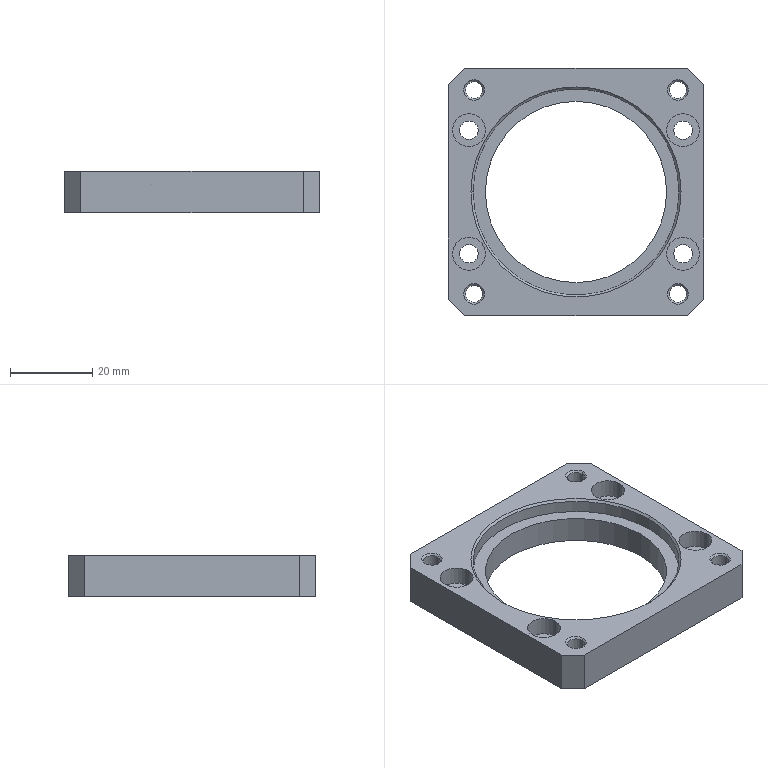Part | STEP file | Guide wheel mechanism revised.sldasm-Part-408 | 1 solid | 61 faces | box 62 x 60 x 10 mm | volume 18303 mm3 | cylinder 28 | cone 18 | plane 15 | commonest cylinder face diameters 4.134 x8 4.5 x8 8 x8 44 x2 50 x2